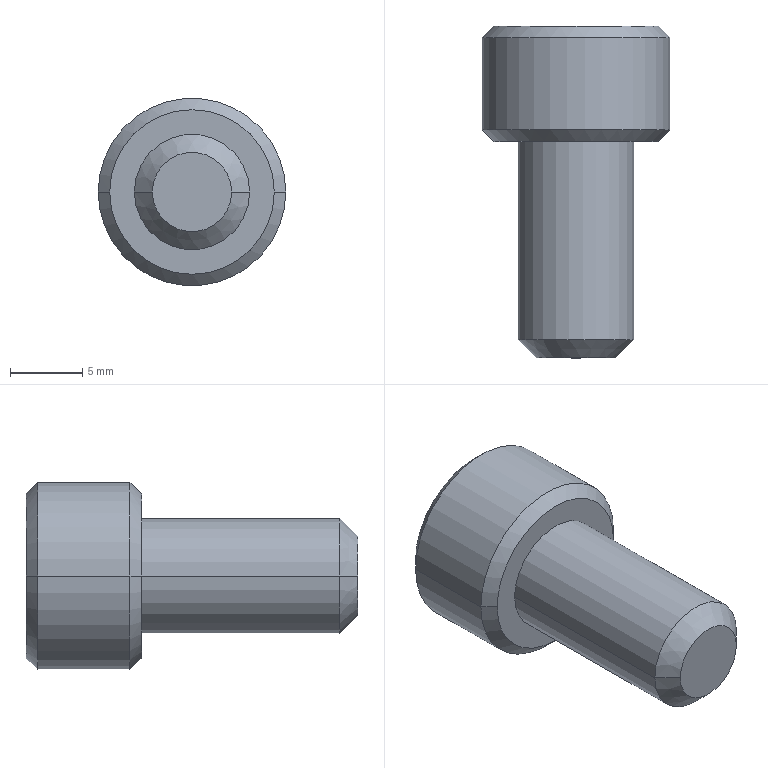Part | STEP file | BB62-M8-15L | 1 solid | 27 faces | box 13 x 23 x 13 mm | volume 1627 mm3 | plane 15 | cone 8 | cylinder 4 | commonest cylinder face diameters 8 x2 13 x2
STEP:
#1=CARTESIAN_POINT('',(0.,2.02,0.));
#2=VERTEX_POINT('',#1);
#3=CARTESIAN_POINT('',(3.43,4.,0.));
#4=VERTEX_POINT('',#3);
#5=CARTESIAN_POINT('',(0.,2.02,0.));
#6=DIRECTION('',(0.866,0.5,0.));
#7=VECTOR('',#6,1000.);
#8=LINE('',#5,#7);
#9=EDGE_CURVE('',#2,#4,#8,.T.);
#10=ORIENTED_EDGE('',*,*,#9,.F.);
#11=CARTESIAN_POINT('',(-3.43,4.,0.));
#12=VERTEX_POINT('',#11);
#13=CARTESIAN_POINT('',(0.,2.02,0.));
#14=DIRECTION('',(-0.866,0.5,0.));
#15=VECTOR('',#14,1000.);
#16=LINE('',#13,#15);
#17=EDGE_CURVE('',#2,#12,#16,.T.);
#18=ORIENTED_EDGE('',*,*,#17,.T.);
#19=CARTESIAN_POINT('',(-2.97,4.,1.715));
#20=VERTEX_POINT('',#19);
#21=CARTESIAN_POINT('',(0.,4.,0.));
#22=DIRECTION('',(0.,-1.,0.));
#23=DIRECTION('',(-1.,0.,0.));
#24=AXIS2_PLACEMENT_3D('',#21,#22,#23);
#25=CIRCLE('',#24,3.43);
#26=EDGE_CURVE('',#20,#12,#25,.T.);
#27=ORIENTED_EDGE('',*,*,#26,.F.);
#28=CARTESIAN_POINT('',(0.,4.,3.43));
#29=VERTEX_POINT('',#28);
#30=CARTESIAN_POINT('',(0.,4.,0.));
#31=DIRECTION('',(0.,-1.,0.));
#32=DIRECTION('',(-1.,0.,0.));
#33=AXIS2_PLACEMENT_3D('',#30,#31,#32);
#34=CIRCLE('',#33,3.43);
#35=EDGE_CURVE('',#29,#20,#34,.T.);
#36=ORIENTED_EDGE('',*,*,#35,.F.);
#37=CARTESIAN_POINT('',(2.97,4.,1.715));
#38=VERTEX_POINT('',#37);
#39=CARTESIAN_POINT('',(0.,4.,0.));
#40=DIRECTION('',(0.,-1.,0.));
#41=DIRECTION('',(-1.,0.,0.));
#42=AXIS2_PLACEMENT_3D('',#39,#40,#41);
#43=CIRCLE('',#42,3.43);
#44=EDGE_CURVE('',#38,#29,#43,.T.);
#45=ORIENTED_EDGE('',*,*,#44,.F.);
#46=CARTESIAN_POINT('',(0.,4.,0.));
#47=DIRECTION('',(0.,-1.,0.));
#48=DIRECTION('',(-1.,0.,0.));
#49=AXIS2_PLACEMENT_3D('',#46,#47,#48);
#50=CIRCLE('',#49,3.43);
#51=EDGE_CURVE('',#4,#38,#50,.T.);
#52=ORIENTED_EDGE('',*,*,#51,.F.);
#53=EDGE_LOOP('',(#10,#18,#27,#36,#45,#52));
#54=FACE_OUTER_BOUND('',#53,.T.);
#55=CARTESIAN_POINT('',(0.,1002.02,0.));
#56=DIRECTION('',(0.,1.,0.));
#57=DIRECTION('',(1.,0.,0.));
#58=AXIS2_PLACEMENT_3D('',#55,#56,#57);
#59=CONICAL_SURFACE('',#58,1732.051,1.047);
#60=ADVANCED_FACE('',(#54),#59,.F.);
#61=CARTESIAN_POINT('',(2.75,-15.,0.));
#62=VERTEX_POINT('',#61);
#63=CARTESIAN_POINT('',(-2.75,-15.,0.));
#64=VERTEX_POINT('',#63);
#65=CARTESIAN_POINT('',(0.,-15.,0.));
#66=DIRECTION('',(0.,1.,0.));
#67=DIRECTION('',(1.,0.,0.));
#68=AXIS2_PLACEMENT_3D('',#65,#66,#67);
#69=CIRCLE('',#68,2.75);
#70=EDGE_CURVE('',#62,#64,#69,.T.);
#71=ORIENTED_EDGE('',*,*,#70,.T.);
#72=CARTESIAN_POINT('',(-4.,-13.75,0.));
#73=VERTEX_POINT('',#72);
#74=CARTESIAN_POINT('',(-2.75,-15.,0.));
#75=DIRECTION('',(-0.7071,0.7071,0.));
#76=VECTOR('',#75,1000.);
#77=LINE('',#74,#76);
#78=EDGE_CURVE('',#64,#73,#77,.T.);
#79=ORIENTED_EDGE('',*,*,#78,.T.);
#80=CARTESIAN_POINT('',(4.,-13.75,0.));
#81=VERTEX_POINT('',#80);
#82=CARTESIAN_POINT('',(0.,-13.75,0.));
#83=DIRECTION('',(0.,-1.,0.));
#84=DIRECTION('',(-1.,0.,0.));
#85=AXIS2_PLACEMENT_3D('',#82,#83,#84);
#86=CIRCLE('',#85,4.);
#87=EDGE_CURVE('',#73,#81,#86,.T.);
#88=ORIENTED_EDGE('',*,*,#87,.T.);
#89=CARTESIAN_POINT('',(2.75,-15.,0.));
#90=DIRECTION('',(0.7071,0.7071,0.));
#91=VECTOR('',#90,1000.);
#92=LINE('',#89,#91);
#93=EDGE_CURVE('',#62,#81,#92,.T.);
#94=ORIENTED_EDGE('',*,*,#93,.F.);
#95=EDGE_LOOP('',(#71,#79,#88,#94));
#96=FACE_OUTER_BOUND('',#95,.T.);
#97=CARTESIAN_POINT('',(0.,-15.,0.));
#98=DIRECTION('',(0.,1.,0.));
#99=DIRECTION('',(1.,0.,0.));
#100=AXIS2_PLACEMENT_3D('',#97,#98,#99);
#101=CONICAL_SURFACE('',#100,2.75,0.7854);
#102=ADVANCED_FACE('',(#96),#101,.T.);
#103=ORIENTED_EDGE('',*,*,#87,.F.);
#104=CARTESIAN_POINT('',(-4.,0.,0.));
#105=VERTEX_POINT('',#104);
#106=CARTESIAN_POINT('',(-4.,-13.75,0.));
#107=DIRECTION('',(0.,1.,0.));
#108=VECTOR('',#107,1000.);
#109=LINE('',#106,#108);
#110=EDGE_CURVE('',#73,#105,#109,.T.);
#111=ORIENTED_EDGE('',*,*,#110,.T.);
#112=CARTESIAN_POINT('',(4.,0.,0.));
#113=VERTEX_POINT('',#112);
#114=CARTESIAN_POINT('',(0.,0.,0.));
#115=DIRECTION('',(0.,-1.,0.));
#116=DIRECTION('',(-1.,0.,0.));
#117=AXIS2_PLACEMENT_3D('',#114,#115,#116);
#118=CIRCLE('',#117,4.);
#119=EDGE_CURVE('',#105,#113,#118,.T.);
#120=ORIENTED_EDGE('',*,*,#119,.T.);
#121=CARTESIAN_POINT('',(4.,-13.75,0.));
#122=DIRECTION('',(0.,1.,0.));
#123=VECTOR('',#122,1000.);
#124=LINE('',#121,#123);
#125=EDGE_CURVE('',#81,#113,#124,.T.);
#126=ORIENTED_EDGE('',*,*,#125,.F.);
#127=EDGE_LOOP('',(#103,#111,#120,#126));
#128=FACE_OUTER_BOUND('',#127,.T.);
#129=CARTESIAN_POINT('',(0.,-13.75,0.));
#130=DIRECTION('',(0.,1.,0.));
#131=DIRECTION('',(1.,0.,0.));
#132=AXIS2_PLACEMENT_3D('',#129,#130,#131);
#133=CYLINDRICAL_SURFACE('',#132,4.);
#134=ADVANCED_FACE('',(#128),#133,.T.);
#135=CARTESIAN_POINT('',(-5.7,8.,0.));
#136=VERTEX_POINT('',#135);
#137=CARTESIAN_POINT('',(5.7,8.,0.));
#138=VERTEX_POINT('',#137);
#139=CARTESIAN_POINT('',(0.,8.,0.));
#140=DIRECTION('',(0.,-1.,0.));
#141=DIRECTION('',(-1.,0.,0.));
#142=AXIS2_PLACEMENT_3D('',#139,#140,#141);
#143=CIRCLE('',#142,5.7);
#144=EDGE_CURVE('',#136,#138,#143,.T.);
#145=ORIENTED_EDGE('',*,*,#144,.T.);
#146=CARTESIAN_POINT('',(6.5,7.2,0.));
#147=VERTEX_POINT('',#146);
#148=CARTESIAN_POINT('',(6.5,7.2,0.));
#149=DIRECTION('',(0.7071,-0.7071,0.));
#150=VECTOR('',#149,1000.);
#151=LINE('',#148,#150);
#152=EDGE_CURVE('',#138,#147,#151,.T.);
#153=ORIENTED_EDGE('',*,*,#152,.T.);
#154=CARTESIAN_POINT('',(-6.5,7.2,0.));
#155=VERTEX_POINT('',#154);
#156=CARTESIAN_POINT('',(0.,7.2,0.));
#157=DIRECTION('',(0.,-1.,0.));
#158=DIRECTION('',(-1.,0.,0.));
#159=AXIS2_PLACEMENT_3D('',#156,#157,#158);
#160=CIRCLE('',#159,6.5);
#161=EDGE_CURVE('',#155,#147,#160,.T.);
#162=ORIENTED_EDGE('',*,*,#161,.F.);
#163=CARTESIAN_POINT('',(-6.5,7.2,0.));
#164=DIRECTION('',(-0.7071,-0.7071,0.));
#165=VECTOR('',#164,1000.);
#166=LINE('',#163,#165);
#167=EDGE_CURVE('',#136,#155,#166,.T.);
#168=ORIENTED_EDGE('',*,*,#167,.F.);
#169=EDGE_LOOP('',(#145,#153,#162,#168));
#170=FACE_OUTER_BOUND('',#169,.T.);
#171=CARTESIAN_POINT('',(0.,7.2,0.));
#172=DIRECTION('',(0.,-1.,0.));
#173=DIRECTION('',(-1.,0.,0.));
#174=AXIS2_PLACEMENT_3D('',#171,#172,#173);
#175=CONICAL_SURFACE('',#174,6.5,0.7854);
#176=ADVANCED_FACE('',(#170),#175,.T.);
#177=ORIENTED_EDGE('',*,*,#161,.T.);
#178=CARTESIAN_POINT('',(6.5,0.8,0.));
#179=VERTEX_POINT('',#178);
#180=CARTESIAN_POINT('',(6.5,1.62,0.));
#181=DIRECTION('',(0.,-1.,0.));
#182=VECTOR('',#181,1000.);
#183=LINE('',#180,#182);
#184=EDGE_CURVE('',#147,#179,#183,.T.);
#185=ORIENTED_EDGE('',*,*,#184,.T.);
#186=CARTESIAN_POINT('',(-6.5,0.8,0.));
#187=VERTEX_POINT('',#186);
#188=CARTESIAN_POINT('',(0.,0.8,0.));
#189=DIRECTION('',(0.,-1.,0.));
#190=DIRECTION('',(-1.,0.,0.));
#191=AXIS2_PLACEMENT_3D('',#188,#189,#190);
#192=CIRCLE('',#191,6.5);
#193=EDGE_CURVE('',#187,#179,#192,.T.);
#194=ORIENTED_EDGE('',*,*,#193,.F.);
#195=CARTESIAN_POINT('',(-6.5,1.62,0.));
#196=DIRECTION('',(0.,-1.,0.));
#197=VECTOR('',#196,1000.);
#198=LINE('',#195,#197);
#199=EDGE_CURVE('',#155,#187,#198,.T.);
#200=ORIENTED_EDGE('',*,*,#199,.F.);
#201=EDGE_LOOP('',(#177,#185,#194,#200));
#202=FACE_OUTER_BOUND('',#201,.T.);
#203=CARTESIAN_POINT('',(0.,1.62,0.));
#204=DIRECTION('',(0.,-1.,0.));
#205=DIRECTION('',(-1.,0.,0.));
#206=AXIS2_PLACEMENT_3D('',#203,#204,#205);
#207=CYLINDRICAL_SURFACE('',#206,6.5);
#208=ADVANCED_FACE('',(#202),#207,.T.);
#209=CARTESIAN_POINT('',(-5.7,0.,0.));
#210=VERTEX_POINT('',#209);
#211=CARTESIAN_POINT('',(5.7,0.,0.));
#212=VERTEX_POINT('',#211);
#213=CARTESIAN_POINT('',(0.,0.,0.));
#214=DIRECTION('',(0.,-1.,0.));
#215=DIRECTION('',(-1.,0.,0.));
#216=AXIS2_PLACEMENT_3D('',#213,#214,#215);
#217=CIRCLE('',#216,5.7);
#218=EDGE_CURVE('',#210,#212,#217,.T.);
#219=ORIENTED_EDGE('',*,*,#218,.F.);
#220=CARTESIAN_POINT('',(-5.7,0.,0.));
#221=DIRECTION('',(-0.7071,0.7071,0.));
#222=VECTOR('',#221,1000.);
#223=LINE('',#220,#222);
#224=EDGE_CURVE('',#210,#187,#223,.T.);
#225=ORIENTED_EDGE('',*,*,#224,.T.);
#226=ORIENTED_EDGE('',*,*,#193,.T.);
#227=CARTESIAN_POINT('',(5.7,0.,0.));
#228=DIRECTION('',(0.7071,0.7071,0.));
#229=VECTOR('',#228,1000.);
#230=LINE('',#227,#229);
#231=EDGE_CURVE('',#212,#179,#230,.T.);
#232=ORIENTED_EDGE('',*,*,#231,.F.);
#233=EDGE_LOOP('',(#219,#225,#226,#232));
#234=FACE_OUTER_BOUND('',#233,.T.);
#235=CARTESIAN_POINT('',(0.,0.,0.));
#236=DIRECTION('',(0.,1.,0.));
#237=DIRECTION('',(1.,0.,0.));
#238=AXIS2_PLACEMENT_3D('',#235,#236,#237);
#239=CONICAL_SURFACE('',#238,5.7,0.7854);
#240=ADVANCED_FACE('',(#234),#239,.T.);
#241=ORIENTED_EDGE('',*,*,#144,.F.);
#242=CARTESIAN_POINT('',(0.,8.,0.));
#243=DIRECTION('',(0.,-1.,0.));
#244=DIRECTION('',(-1.,0.,0.));
#245=AXIS2_PLACEMENT_3D('',#242,#243,#244);
#246=CIRCLE('',#245,5.7);
#247=EDGE_CURVE('',#138,#136,#246,.T.);
#248=ORIENTED_EDGE('',*,*,#247,.F.);
#249=EDGE_LOOP('',(#241,#248));
#250=FACE_OUTER_BOUND('',#249,.T.);
#251=CARTESIAN_POINT('',(0.,8.,-3.43));
#252=VERTEX_POINT('',#251);
#253=CARTESIAN_POINT('',(-2.97,8.,-1.715));
#254=VERTEX_POINT('',#253);
#255=CARTESIAN_POINT('',(0.,8.,-3.43));
#256=DIRECTION('',(-0.866,0.,0.5));
#257=VECTOR('',#256,1000.);
#258=LINE('',#255,#257);
#259=EDGE_CURVE('',#252,#254,#258,.T.);
#260=ORIENTED_EDGE('',*,*,#259,.F.);
#261=CARTESIAN_POINT('',(2.97,8.,-1.715));
#262=VERTEX_POINT('',#261);
#263=CARTESIAN_POINT('',(2.97,8.,-1.715));
#264=DIRECTION('',(-0.866,0.,-0.5));
#265=VECTOR('',#264,1000.);
#266=LINE('',#263,#265);
#267=EDGE_CURVE('',#262,#252,#266,.T.);
#268=ORIENTED_EDGE('',*,*,#267,.F.);
#269=CARTESIAN_POINT('',(2.97,8.,1.715));
#270=VERTEX_POINT('',#269);
#271=CARTESIAN_POINT('',(2.97,8.,1.715));
#272=DIRECTION('',(0.,0.,-1.));
#273=VECTOR('',#272,1000.);
#274=LINE('',#271,#273);
#275=EDGE_CURVE('',#270,#262,#274,.T.);
#276=ORIENTED_EDGE('',*,*,#275,.F.);
#277=CARTESIAN_POINT('',(0.,8.,3.43));
#278=VERTEX_POINT('',#277);
#279=CARTESIAN_POINT('',(0.,8.,3.43));
#280=DIRECTION('',(0.866,0.,-0.5));
#281=VECTOR('',#280,1000.);
#282=LINE('',#279,#281);
#283=EDGE_CURVE('',#278,#270,#282,.T.);
#284=ORIENTED_EDGE('',*,*,#283,.F.);
#285=CARTESIAN_POINT('',(-2.97,8.,1.715));
#286=VERTEX_POINT('',#285);
#287=CARTESIAN_POINT('',(-2.97,8.,1.715));
#288=DIRECTION('',(0.866,0.,0.5));
#289=VECTOR('',#288,1000.);
#290=LINE('',#287,#289);
#291=EDGE_CURVE('',#286,#278,#290,.T.);
#292=ORIENTED_EDGE('',*,*,#291,.F.);
#293=CARTESIAN_POINT('',(-2.97,8.,-1.715));
#294=DIRECTION('',(0.,0.,1.));
#295=VECTOR('',#294,1000.);
#296=LINE('',#293,#295);
#297=EDGE_CURVE('',#254,#286,#296,.T.);
#298=ORIENTED_EDGE('',*,*,#297,.F.);
#299=EDGE_LOOP('',(#260,#268,#276,#284,#292,#298));
#300=FACE_BOUND('',#299,.T.);
#301=CARTESIAN_POINT('',(5.7,8.,0.));
#302=DIRECTION('',(0.,1.,0.));
#303=DIRECTION('',(1.,0.,0.));
#304=AXIS2_PLACEMENT_3D('',#301,#302,#303);
#305=PLANE('',#304);
#306=ADVANCED_FACE('',(#250,#300),#305,.T.);
#307=CARTESIAN_POINT('',(0.,0.,0.));
#308=DIRECTION('',(0.,-1.,0.));
#309=DIRECTION('',(-1.,0.,0.));
#310=AXIS2_PLACEMENT_3D('',#307,#308,#309);
#311=CIRCLE('',#310,4.);
#312=EDGE_CURVE('',#113,#105,#311,.T.);
#313=ORIENTED_EDGE('',*,*,#312,.F.);
#314=ORIENTED_EDGE('',*,*,#119,.F.);
#315=EDGE_LOOP('',(#313,#314));
#316=FACE_BOUND('',#315,.T.);
#317=CARTESIAN_POINT('',(0.,0.,0.));
#318=DIRECTION('',(0.,-1.,0.));
#319=DIRECTION('',(-1.,0.,0.));
#320=AXIS2_PLACEMENT_3D('',#317,#318,#319);
#321=CIRCLE('',#320,5.7);
#322=EDGE_CURVE('',#212,#210,#321,.T.);
#323=ORIENTED_EDGE('',*,*,#322,.T.);
#324=ORIENTED_EDGE('',*,*,#218,.T.);
#325=EDGE_LOOP('',(#323,#324));
#326=FACE_OUTER_BOUND('',#325,.T.);
#327=CARTESIAN_POINT('',(0.,0.,0.));
#328=DIRECTION('',(0.,-1.,0.));
#329=DIRECTION('',(-1.,0.,0.));
#330=AXIS2_PLACEMENT_3D('',#327,#328,#329);
#331=PLANE('',#330);
#332=ADVANCED_FACE('',(#316,#326),#331,.T.);
#333=ORIENTED_EDGE('',*,*,#224,.F.);
#334=ORIENTED_EDGE('',*,*,#322,.F.);
#335=ORIENTED_EDGE('',*,*,#231,.T.);
#336=CARTESIAN_POINT('',(0.,0.8,0.));
#337=DIRECTION('',(0.,-1.,0.));
#338=DIRECTION('',(-1.,0.,0.));
#339=AXIS2_PLACEMENT_3D('',#336,#337,#338);
#340=CIRCLE('',#339,6.5);
#341=EDGE_CURVE('',#179,#187,#340,.T.);
#342=ORIENTED_EDGE('',*,*,#341,.T.);
#343=EDGE_LOOP('',(#333,#334,#335,#342));
#344=FACE_OUTER_BOUND('',#343,.T.);
#345=CARTESIAN_POINT('',(0.,0.,0.));
#346=DIRECTION('',(0.,1.,0.));
#347=DIRECTION('',(1.,0.,0.));
#348=AXIS2_PLACEMENT_3D('',#345,#346,#347);
#349=CONICAL_SURFACE('',#348,5.7,0.7854);
#350=ADVANCED_FACE('',(#344),#349,.T.);
#351=ORIENTED_EDGE('',*,*,#184,.F.);
#352=CARTESIAN_POINT('',(0.,7.2,0.));
#353=DIRECTION('',(0.,-1.,0.));
#354=DIRECTION('',(-1.,0.,0.));
#355=AXIS2_PLACEMENT_3D('',#352,#353,#354);
#356=CIRCLE('',#355,6.5);
#357=EDGE_CURVE('',#147,#155,#356,.T.);
#358=ORIENTED_EDGE('',*,*,#357,.T.);
#359=ORIENTED_EDGE('',*,*,#199,.T.);
#360=ORIENTED_EDGE('',*,*,#341,.F.);
#361=EDGE_LOOP('',(#351,#358,#359,#360));
#362=FACE_OUTER_BOUND('',#361,.T.);
#363=CARTESIAN_POINT('',(0.,1.62,0.));
#364=DIRECTION('',(0.,-1.,0.));
#365=DIRECTION('',(-1.,0.,0.));
#366=AXIS2_PLACEMENT_3D('',#363,#364,#365);
#367=CYLINDRICAL_SURFACE('',#366,6.5);
#368=ADVANCED_FACE('',(#362),#367,.T.);
#369=ORIENTED_EDGE('',*,*,#152,.F.);
#370=ORIENTED_EDGE('',*,*,#247,.T.);
#371=ORIENTED_EDGE('',*,*,#167,.T.);
#372=ORIENTED_EDGE('',*,*,#357,.F.);
#373=EDGE_LOOP('',(#369,#370,#371,#372));
#374=FACE_OUTER_BOUND('',#373,.T.);
#375=CARTESIAN_POINT('',(0.,7.2,0.));
#376=DIRECTION('',(0.,-1.,0.));
#377=DIRECTION('',(-1.,0.,0.));
#378=AXIS2_PLACEMENT_3D('',#375,#376,#377);
#379=CONICAL_SURFACE('',#378,6.5,0.7854);
#380=ADVANCED_FACE('',(#374),#379,.T.);
#381=ORIENTED_EDGE('',*,*,#110,.F.);
#382=CARTESIAN_POINT('',(0.,-13.75,0.));
#383=DIRECTION('',(0.,-1.,0.));
#384=DIRECTION('',(-1.,0.,0.));
#385=AXIS2_PLACEMENT_3D('',#382,#383,#384);
#386=CIRCLE('',#385,4.);
#387=EDGE_CURVE('',#81,#73,#386,.T.);
#388=ORIENTED_EDGE('',*,*,#387,.F.);
#389=ORIENTED_EDGE('',*,*,#125,.T.);
#390=ORIENTED_EDGE('',*,*,#312,.T.);
#391=EDGE_LOOP('',(#381,#388,#389,#390));
#392=FACE_OUTER_BOUND('',#391,.T.);
#393=CARTESIAN_POINT('',(0.,-13.75,0.));
#394=DIRECTION('',(0.,1.,0.));
#395=DIRECTION('',(1.,0.,0.));
#396=AXIS2_PLACEMENT_3D('',#393,#394,#395);
#397=CYLINDRICAL_SURFACE('',#396,4.);
#398=ADVANCED_FACE('',(#392),#397,.T.);
#399=ORIENTED_EDGE('',*,*,#70,.F.);
#400=CARTESIAN_POINT('',(0.,-15.,0.));
#401=DIRECTION('',(0.,1.,0.));
#402=DIRECTION('',(1.,0.,0.));
#403=AXIS2_PLACEMENT_3D('',#400,#401,#402);
#404=CIRCLE('',#403,2.75);
#405=EDGE_CURVE('',#64,#62,#404,.T.);
#406=ORIENTED_EDGE('',*,*,#405,.F.);
#407=EDGE_LOOP('',(#399,#406));
#408=FACE_OUTER_BOUND('',#407,.T.);
#409=CARTESIAN_POINT('',(0.,-15.,0.));
#410=DIRECTION('',(0.,-1.,0.));
#411=DIRECTION('',(-1.,0.,0.));
#412=AXIS2_PLACEMENT_3D('',#409,#410,#411);
#413=PLANE('',#412);
#414=ADVANCED_FACE('',(#408),#413,.T.);
#415=ORIENTED_EDGE('',*,*,#78,.F.);
#416=ORIENTED_EDGE('',*,*,#405,.T.);
#417=ORIENTED_EDGE('',*,*,#93,.T.);
#418=ORIENTED_EDGE('',*,*,#387,.T.);
#419=EDGE_LOOP('',(#415,#416,#417,#418));
#420=FACE_OUTER_BOUND('',#419,.T.);
#421=CARTESIAN_POINT('',(0.,-15.,0.));
#422=DIRECTION('',(0.,1.,0.));
#423=DIRECTION('',(1.,0.,0.));
#424=AXIS2_PLACEMENT_3D('',#421,#422,#423);
#425=CONICAL_SURFACE('',#424,2.75,0.7854);
#426=ADVANCED_FACE('',(#420),#425,.T.);
#427=CARTESIAN_POINT('',(2.97,4.,-1.715));
#428=VERTEX_POINT('',#427);
#429=CARTESIAN_POINT('',(0.,4.,-3.43));
#430=VERTEX_POINT('',#429);
#431=CARTESIAN_POINT('',(2.97,4.,-1.715));
#432=DIRECTION('',(-0.866,0.,-0.5));
#433=VECTOR('',#432,1000.);
#434=LINE('',#431,#433);
#435=EDGE_CURVE('',#428,#430,#434,.T.);
#436=ORIENTED_EDGE('',*,*,#435,.F.);
#437=CARTESIAN_POINT('',(2.97,8.,-1.715));
#438=DIRECTION('',(0.,-1.,0.));
#439=VECTOR('',#438,1000.);
#440=LINE('',#437,#439);
#441=EDGE_CURVE('',#262,#428,#440,.T.);
#442=ORIENTED_EDGE('',*,*,#441,.F.);
#443=ORIENTED_EDGE('',*,*,#267,.T.);
#444=CARTESIAN_POINT('',(0.,8.,-3.43));
#445=DIRECTION('',(0.,-1.,0.));
#446=VECTOR('',#445,1000.);
#447=LINE('',#444,#446);
#448=EDGE_CURVE('',#252,#430,#447,.T.);
#449=ORIENTED_EDGE('',*,*,#448,.T.);
#450=EDGE_LOOP('',(#436,#442,#443,#449));
#451=FACE_OUTER_BOUND('',#450,.T.);
#452=CARTESIAN_POINT('',(2.97,8.,-1.715));
#453=DIRECTION('',(-0.5,0.,0.866));
#454=DIRECTION('',(0.866,0.,0.5));
#455=AXIS2_PLACEMENT_3D('',#452,#453,#454);
#456=PLANE('',#455);
#457=ADVANCED_FACE('',(#451),#456,.T.);
#458=CARTESIAN_POINT('',(-2.97,4.,-1.715));
#459=VERTEX_POINT('',#458);
#460=CARTESIAN_POINT('',(0.,4.,-3.43));
#461=DIRECTION('',(-0.866,0.,0.5));
#462=VECTOR('',#461,1000.);
#463=LINE('',#460,#462);
#464=EDGE_CURVE('',#430,#459,#463,.T.);
#465=ORIENTED_EDGE('',*,*,#464,.F.);
#466=ORIENTED_EDGE('',*,*,#448,.F.);
#467=ORIENTED_EDGE('',*,*,#259,.T.);
#468=CARTESIAN_POINT('',(-2.97,8.,-1.715));
#469=DIRECTION('',(0.,-1.,0.));
#470=VECTOR('',#469,1000.);
#471=LINE('',#468,#470);
#472=EDGE_CURVE('',#254,#459,#471,.T.);
#473=ORIENTED_EDGE('',*,*,#472,.T.);
#474=EDGE_LOOP('',(#465,#466,#467,#473));
#475=FACE_OUTER_BOUND('',#474,.T.);
#476=CARTESIAN_POINT('',(0.,8.,-3.43));
#477=DIRECTION('',(0.5,0.,0.866));
#478=DIRECTION('',(0.866,0.,-0.5));
#479=AXIS2_PLACEMENT_3D('',#476,#477,#478);
#480=PLANE('',#479);
#481=ADVANCED_FACE('',(#475),#480,.T.);
#482=CARTESIAN_POINT('',(-2.97,4.,-1.715));
#483=DIRECTION('',(0.,0.,1.));
#484=VECTOR('',#483,1000.);
#485=LINE('',#482,#484);
#486=EDGE_CURVE('',#459,#20,#485,.T.);
#487=ORIENTED_EDGE('',*,*,#486,.F.);
#488=ORIENTED_EDGE('',*,*,#472,.F.);
#489=ORIENTED_EDGE('',*,*,#297,.T.);
#490=CARTESIAN_POINT('',(-2.97,8.,1.715));
#491=DIRECTION('',(0.,-1.,0.));
#492=VECTOR('',#491,1000.);
#493=LINE('',#490,#492);
#494=EDGE_CURVE('',#286,#20,#493,.T.);
#495=ORIENTED_EDGE('',*,*,#494,.T.);
#496=EDGE_LOOP('',(#487,#488,#489,#495));
#497=FACE_OUTER_BOUND('',#496,.T.);
#498=CARTESIAN_POINT('',(-2.97,8.,-1.715));
#499=DIRECTION('',(1.,0.,0.));
#500=DIRECTION('',(0.,0.,-1.));
#501=AXIS2_PLACEMENT_3D('',#498,#499,#500);
#502=PLANE('',#501);
#503=ADVANCED_FACE('',(#497),#502,.T.);
#504=CARTESIAN_POINT('',(-2.97,4.,1.715));
#505=DIRECTION('',(0.866,0.,0.5));
#506=VECTOR('',#505,1000.);
#507=LINE('',#504,#506);
#508=EDGE_CURVE('',#20,#29,#507,.T.);
#509=ORIENTED_EDGE('',*,*,#508,.F.);
#510=ORIENTED_EDGE('',*,*,#494,.F.);
#511=ORIENTED_EDGE('',*,*,#291,.T.);
#512=CARTESIAN_POINT('',(0.,8.,3.43));
#513=DIRECTION('',(0.,-1.,0.));
#514=VECTOR('',#513,1000.);
#515=LINE('',#512,#514);
#516=EDGE_CURVE('',#278,#29,#515,.T.);
#517=ORIENTED_EDGE('',*,*,#516,.T.);
#518=EDGE_LOOP('',(#509,#510,#511,#517));
#519=FACE_OUTER_BOUND('',#518,.T.);
#520=CARTESIAN_POINT('',(-2.97,8.,1.715));
#521=DIRECTION('',(0.5,0.,-0.866));
#522=DIRECTION('',(-0.866,0.,-0.5));
#523=AXIS2_PLACEMENT_3D('',#520,#521,#522);
#524=PLANE('',#523);
#525=ADVANCED_FACE('',(#519),#524,.T.);
#526=CARTESIAN_POINT('',(0.,4.,3.43));
#527=DIRECTION('',(0.866,0.,-0.5));
#528=VECTOR('',#527,1000.);
#529=LINE('',#526,#528);
#530=EDGE_CURVE('',#29,#38,#529,.T.);
#531=ORIENTED_EDGE('',*,*,#530,.F.);
#532=ORIENTED_EDGE('',*,*,#516,.F.);
#533=ORIENTED_EDGE('',*,*,#283,.T.);
#534=CARTESIAN_POINT('',(2.97,8.,1.715));
#535=DIRECTION('',(0.,-1.,0.));
#536=VECTOR('',#535,1000.);
#537=LINE('',#534,#536);
#538=EDGE_CURVE('',#270,#38,#537,.T.);
#539=ORIENTED_EDGE('',*,*,#538,.T.);
#540=EDGE_LOOP('',(#531,#532,#533,#539));
#541=FACE_OUTER_BOUND('',#540,.T.);
#542=CARTESIAN_POINT('',(0.,8.,3.43));
#543=DIRECTION('',(-0.5,0.,-0.866));
#544=DIRECTION('',(-0.866,0.,0.5));
#545=AXIS2_PLACEMENT_3D('',#542,#543,#544);
#546=PLANE('',#545);
#547=ADVANCED_FACE('',(#541),#546,.T.);
#548=CARTESIAN_POINT('',(2.97,4.,1.715));
#549=DIRECTION('',(0.,0.,-1.));
#550=VECTOR('',#549,1000.);
#551=LINE('',#548,#550);
#552=EDGE_CURVE('',#38,#428,#551,.T.);
#553=ORIENTED_EDGE('',*,*,#552,.F.);
#554=ORIENTED_EDGE('',*,*,#538,.F.);
#555=ORIENTED_EDGE('',*,*,#275,.T.);
#556=ORIENTED_EDGE('',*,*,#441,.T.);
#557=EDGE_LOOP('',(#553,#554,#555,#556));
#558=FACE_OUTER_BOUND('',#557,.T.);
#559=CARTESIAN_POINT('',(2.97,8.,1.715));
#560=DIRECTION('',(-1.,0.,0.));
#561=DIRECTION('',(0.,0.,1.));
#562=AXIS2_PLACEMENT_3D('',#559,#560,#561);
#563=PLANE('',#562);
#564=ADVANCED_FACE('',(#558),#563,.T.);
#565=ORIENTED_EDGE('',*,*,#435,.T.);
#566=CARTESIAN_POINT('',(0.,4.,0.));
#567=DIRECTION('',(0.,-1.,0.));
#568=DIRECTION('',(-1.,0.,0.));
#569=AXIS2_PLACEMENT_3D('',#566,#567,#568);
#570=CIRCLE('',#569,3.43);
#571=EDGE_CURVE('',#430,#428,#570,.T.);
#572=ORIENTED_EDGE('',*,*,#571,.T.);
#573=EDGE_LOOP('',(#565,#572));
#574=FACE_OUTER_BOUND('',#573,.T.);
#575=CARTESIAN_POINT('',(0.,4.,0.));
#576=DIRECTION('',(0.,1.,0.));
#577=DIRECTION('',(1.,0.,0.));
#578=AXIS2_PLACEMENT_3D('',#575,#576,#577);
#579=PLANE('',#578);
#580=ADVANCED_FACE('',(#574),#579,.F.);
#581=ORIENTED_EDGE('',*,*,#552,.T.);
#582=CARTESIAN_POINT('',(0.,4.,0.));
#583=DIRECTION('',(0.,-1.,0.));
#584=DIRECTION('',(-1.,0.,0.));
#585=AXIS2_PLACEMENT_3D('',#582,#583,#584);
#586=CIRCLE('',#585,3.43);
#587=EDGE_CURVE('',#428,#4,#586,.T.);
#588=ORIENTED_EDGE('',*,*,#587,.T.);
#589=ORIENTED_EDGE('',*,*,#51,.T.);
#590=EDGE_LOOP('',(#581,#588,#589));
#591=FACE_OUTER_BOUND('',#590,.T.);
#592=CARTESIAN_POINT('',(0.,4.,0.));
#593=DIRECTION('',(0.,1.,0.));
#594=DIRECTION('',(1.,0.,0.));
#595=AXIS2_PLACEMENT_3D('',#592,#593,#594);
#596=PLANE('',#595);
#597=ADVANCED_FACE('',(#591),#596,.F.);
#598=ORIENTED_EDGE('',*,*,#530,.T.);
#599=ORIENTED_EDGE('',*,*,#44,.T.);
#600=EDGE_LOOP('',(#598,#599));
#601=FACE_OUTER_BOUND('',#600,.T.);
#602=CARTESIAN_POINT('',(0.,4.,0.));
#603=DIRECTION('',(0.,1.,0.));
#604=DIRECTION('',(1.,0.,0.));
#605=AXIS2_PLACEMENT_3D('',#602,#603,#604);
#606=PLANE('',#605);
#607=ADVANCED_FACE('',(#601),#606,.F.);
#608=ORIENTED_EDGE('',*,*,#508,.T.);
#609=ORIENTED_EDGE('',*,*,#35,.T.);
#610=EDGE_LOOP('',(#608,#609));
#611=FACE_OUTER_BOUND('',#610,.T.);
#612=CARTESIAN_POINT('',(0.,4.,0.));
#613=DIRECTION('',(0.,1.,0.));
#614=DIRECTION('',(1.,0.,0.));
#615=AXIS2_PLACEMENT_3D('',#612,#613,#614);
#616=PLANE('',#615);
#617=ADVANCED_FACE('',(#611),#616,.F.);
#618=ORIENTED_EDGE('',*,*,#486,.T.);
#619=ORIENTED_EDGE('',*,*,#26,.T.);
#620=CARTESIAN_POINT('',(0.,4.,0.));
#621=DIRECTION('',(0.,-1.,0.));
#622=DIRECTION('',(-1.,0.,0.));
#623=AXIS2_PLACEMENT_3D('',#620,#621,#622);
#624=CIRCLE('',#623,3.43);
#625=EDGE_CURVE('',#12,#459,#624,.T.);
#626=ORIENTED_EDGE('',*,*,#625,.T.);
#627=EDGE_LOOP('',(#618,#619,#626));
#628=FACE_OUTER_BOUND('',#627,.T.);
#629=CARTESIAN_POINT('',(0.,4.,0.));
#630=DIRECTION('',(0.,1.,0.));
#631=DIRECTION('',(1.,0.,0.));
#632=AXIS2_PLACEMENT_3D('',#629,#630,#631);
#633=PLANE('',#632);
#634=ADVANCED_FACE('',(#628),#633,.F.);
#635=ORIENTED_EDGE('',*,*,#464,.T.);
#636=CARTESIAN_POINT('',(0.,4.,0.));
#637=DIRECTION('',(0.,-1.,0.));
#638=DIRECTION('',(-1.,0.,0.));
#639=AXIS2_PLACEMENT_3D('',#636,#637,#638);
#640=CIRCLE('',#639,3.43);
#641=EDGE_CURVE('',#459,#430,#640,.T.);
#642=ORIENTED_EDGE('',*,*,#641,.T.);
#643=EDGE_LOOP('',(#635,#642));
#644=FACE_OUTER_BOUND('',#643,.T.);
#645=CARTESIAN_POINT('',(0.,4.,0.));
#646=DIRECTION('',(0.,1.,0.));
#647=DIRECTION('',(1.,0.,0.));
#648=AXIS2_PLACEMENT_3D('',#645,#646,#647);
#649=PLANE('',#648);
#650=ADVANCED_FACE('',(#644),#649,.F.);
#651=ORIENTED_EDGE('',*,*,#17,.F.);
#652=ORIENTED_EDGE('',*,*,#9,.T.);
#653=ORIENTED_EDGE('',*,*,#587,.F.);
#654=ORIENTED_EDGE('',*,*,#571,.F.);
#655=ORIENTED_EDGE('',*,*,#641,.F.);
#656=ORIENTED_EDGE('',*,*,#625,.F.);
#657=EDGE_LOOP('',(#651,#652,#653,#654,#655,#656));
#658=FACE_OUTER_BOUND('',#657,.T.);
#659=CARTESIAN_POINT('',(0.,1002.02,0.));
#660=DIRECTION('',(0.,1.,0.));
#661=DIRECTION('',(1.,0.,0.));
#662=AXIS2_PLACEMENT_3D('',#659,#660,#661);
#663=CONICAL_SURFACE('',#662,1732.051,1.047);
#664=ADVANCED_FACE('',(#658),#663,.F.);
#665=CLOSED_SHELL('',(#60,#102,#134,#176,#208,#240,#306,#332,#350,#368,#380,#398,#414,#426,#457,#481,#503,#525,#547,#564,#580,#597,#607,#617,#634,#650,#664));
#666=MANIFOLD_SOLID_BREP('',#665);
#667=CARTESIAN_POINT('',(0.,0.,0.));
#668=DIRECTION('',(0.,0.,1.));
#669=DIRECTION('',(1.,0.,0.));
#670=AXIS2_PLACEMENT_3D('',#667,#668,#669);
#671=(LENGTH_UNIT()NAMED_UNIT(*)SI_UNIT(.MILLI.,.METRE.));
#672=UNCERTAINTY_MEASURE_WITH_UNIT(LENGTH_MEASURE(0.00001),#671,'','');
#673=(NAMED_UNIT(*)PLANE_ANGLE_UNIT()SI_UNIT($,.RADIAN.));
#674=(NAMED_UNIT(*)SI_UNIT($,.STERADIAN.)SOLID_ANGLE_UNIT());
#675=(GEOMETRIC_REPRESENTATION_CONTEXT(3)GLOBAL_UNCERTAINTY_ASSIGNED_CONTEXT((#672))GLOBAL_UNIT_ASSIGNED_CONTEXT((#671,#673,#674))REPRESENTATION_CONTEXT('',''));
#676=ADVANCED_BREP_SHAPE_REPRESENTATION('',(#666,#670),#675);